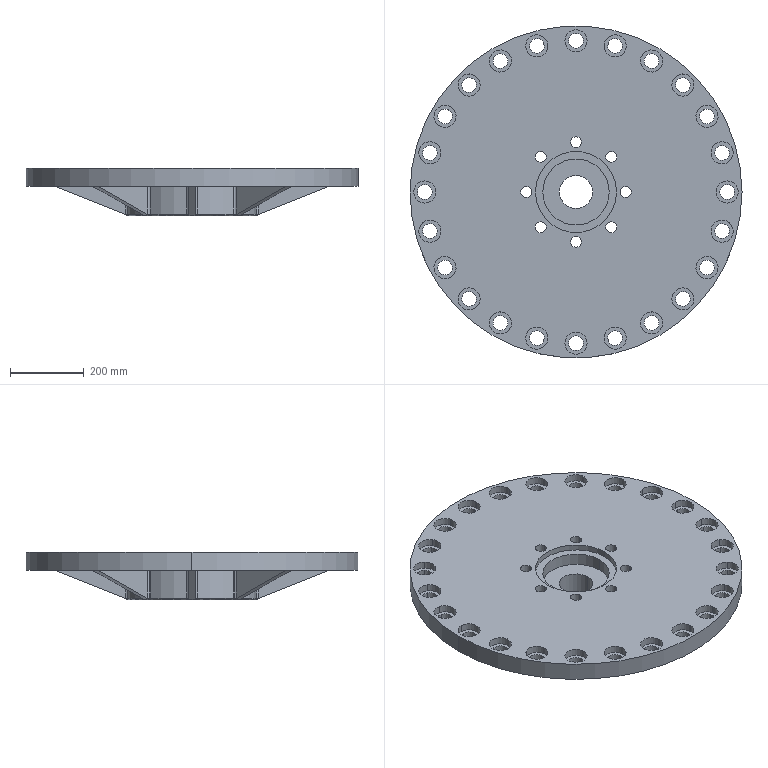Part | SolidWorks | features ICE 6, CirPattern 2, Fillet 2, Extrusion 1, HoleWzd 1 | 1 solid | 217 faces | box 900 x 900 x 130 mm | volume 35744082 mm3 | cylinder 146 | plane 53 | spline 16 | torus 2 | commonest cylinder face diameters 40 x48 60 x48 10 x18 30 x16 350 x8 90 x2